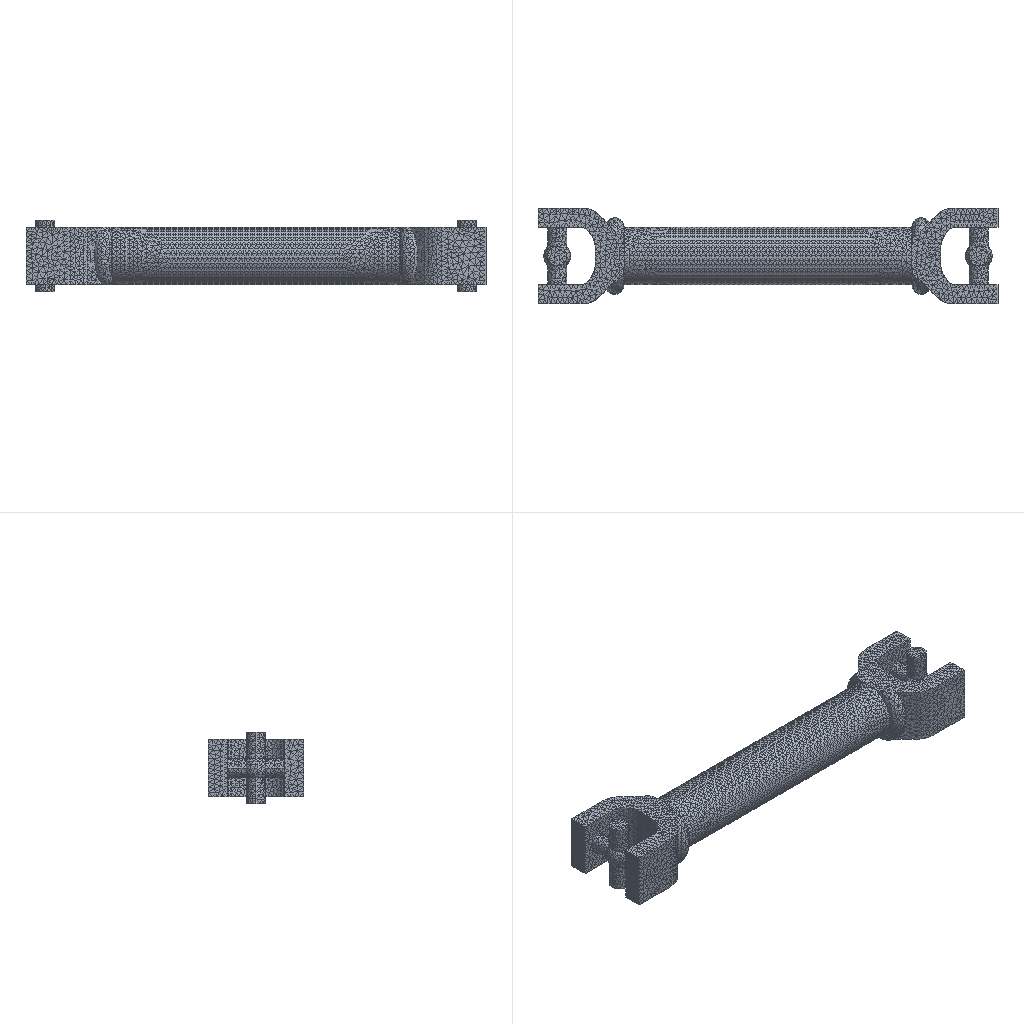Simulation study | ansys workbench
Set-up summary:
category,name,step,type,value,unit,region
solver,ansys_workbench
units,mm-N-s-tonne (MPa),,stated,"/units,MPA"
analysis,LS1,,modal,method=lanb; n_modes=10
load_step,LS1,LS1,modal
mesh,nodes,,,90919
mesh,elements,,,60202
element_type,SOLID187,,,58650
element_type,CONTA174,,,832
element_type,TARGE170,,,720
material,?,,E,240000,tonne s^-2 mm^-1
material,?,,nu,0.3
material,?,,density,6.9e-09,tonne mm^-3
material,16Mn?,,E,210000,tonne s^-2 mm^-1
material,16Mn?,,nu,0.3
material,16Mn?,,density,7.9e-09,tonne mm^-3
bc,Construct Remote Displacement,model,fixed,"[dofs=ROTX,ROTY,ROTZ,UX,UY,UZ n=12]",,node list
contact,Contact Region,,bonded (always),element=CONTA174
contact,Contact Region 2,,bonded (always),element=CONTA174
contact,contact 3,,bonded (always),element=CONTA174
contact,contact 4,,bonded (always),element=CONTA174
named_set,REMOTEDISPALL,,node,2
Ansys APDL input file, long lists of numbers shortened:
/batch
/config,noeldb,1     ! force off writing results to database
*get,_wallstrt,active,,time,wall
! ANSYS input file written by Workbench version 2021 R1
! File used for geometry attach:
/title,______--__ (C5)
! ****** Begin Custom Load Command Snippet ******
/COM, ACT Extensions:
/COM,     LSDYNA, 2021.1
/COM,
! ****** End   Custom Load Command Snippet ******
*DIM,_wb_ProjectScratch_dir,string,248
_wb_ProjectScratch_dir(1) = ''
*DIM,_wb_SolverFiles_dir,string,248
_wb_SolverFiles_dir(1) = ''
*DIM,_wb_userfiles_dir,string,248
_wb_userfiles_dir(1) = ''
/com,--- Data in consistent NMM units. See Solving Units in the help system for more information.
/units,MPA
/nopr
/wb,file,start              !  signify a WB generated input file
/prep7
! Turn off shape checking because checks already performed inside WB mesher.
! See help system for more information.
SHPP,OFF,,NOWARN
/nolist
etcon,set             ! allow ANSYS to choose best KEYOP's for 180x elements, resets any applicable keyopt to MAPDL defaults
/com,*********** Nodes for the whole assembly ***********
nblock,3,,100006
(1i9,3e20.9e3)
        1     7.600000000E+02    -2.000000000E+01     0.000000000E+00
! (90914 more lines like these left out)
-1
/com,*********** Nodes for all Remote Points ***********
nblock,3
(1i9,3e20.9e3)
    90916     7.400000000E+02     1.554312234E-14    -5.712370230E-07
    90917    -1.400000000E+02     1.402403685E-14    -1.421085472E-14
    90918     7.400000000E+02     1.402403685E-14     0.000000000E+00
    90919     7.400000000E+02     1.402403685E-14     0.000000000E+00
-1
/wb,elem,start            !  set before creation of elements
/com,*********** Elements for Body 1 "______|____2" ***********
et,1,187
eblock,19,solid,,52806
(19i9)
        1        1        1        1        0        0        0        0       10        0     5845    15480    21320    15698    17453    58957    61010    58952    58954
! (105611 more lines like these left out)
-1
/com,*********** Elements for Body 2 "______-0|____4" ***********
et,2,187
eblock,19,solid,,2922
(19i9)
        2        2        2        2        0        0        0        0       10        0     2923     5070     5085     5619     5377     6980     7061     6983     6981
! (5843 more lines like these left out)
-1
/com,*********** Elements for Body 3 "______-0|____4[2]" ***********
et,3,187
eblock,19,solid,,2922
(19i9)
        3        3        3        3        0        0        0        0       10        0        1      199      214      748      506     2109     2190     2112     2110
! (5843 more lines like these left out)
-1
/wb,elem,end               !  done creating elements
/com,*********** Send User Defined Coordinate System(s) ***********
csys,0
toffst,273.15,  ! Temperature offset from absolute zero
/com,*********** Set Reference Temperature ***********
tref,22.
/wb,mat,start              !  starting to send materials
/com,*********** Send Materials ***********
MP,DENS,1,6.9e-09,	! tonne mm^-3
MP,EX,1,240000,	! tonne s^-2 mm^-1
MP,NUXY,1,0.3,
MP,DENS,2,7.9e-09,	! tonne mm^-3
MP,EX,2,210000,	! tonne s^-2 mm^-1
MP,NUXY,2,0.3,
MP,DENS,3,7.9e-09,	! tonne mm^-3
MP,EX,3,210000,	! tonne s^-2 mm^-1
MP,NUXY,3,0.3,
/wb,mat,end                !  done sending materials
!************************* Model Summary ********************
!______|____2,	碳纤维合金钢,	matid,	1
!______-0|____4,	16Mn低合金钢,	matid,	2
!______-0|____4[2],	16Mn低合金钢,	matid,	3
!************************* End Model Summary ********************
! get the diagonal of the bounding box. Needed later for other things
*get,_xmin,node,,mnloc,x
*get,_ymin,node,,mnloc,y
*get,_zmin,node,,mnloc,z
*get,_xmax,node,,mxloc,x
*get,_ymax,node,,mxloc,y
*get,_zmax,node,,mxloc,z
_ASMDIAG=(_xmax-_xmin)*(_xmax-_xmin)+(_ymax-_ymin)*(_ymax-_ymin)+(_zmax-_zmin)*(_zmax-_zmin)
_ASMDIAG=SQRT(_ASMDIAG)
/wb,contact,start          !  starting to send contact
/com,*********** Create Contact "接触区域" ***********
/com,            Real Constant Set For Above Contact Is 5 & 4
*set,tid,5
*set,cid,4
r,tid
r,cid
et,tid,170
et,cid,174
eblock,10,,,160
(15i9)
    70895        5        5        5        0     9779     9788     9781     9781    21636    21646     9781    21635
! (159 more lines like these left out)
-1
eblock,10,,,160
(15i9)
    71055        4        4        4        0     9779     9788     9781     9781    21636    21646     9781    21635
! (159 more lines like these left out)
-1
eblock,10,,,200
(15i9)
    71215        4        5        4        0     4877     4884     4882     4882     5669     5706     4882     5668
! (199 more lines like these left out)
-1
eblock,10,,,200
(15i9)
    71415        5        4        5        0     4877     4884     4882     4882     5669     5706     4882     5668
! (199 more lines like these left out)
-1
keyo,cid,8,2               ! auto create asymmetric contact (from Program Controlled setting)
keyo,cid,10,0              ! adjust contact stiffness each NR iteration (from Program Controlled setting)
keyo,cid,12,5              ! bonded always
keyo,cid,18,1              ! small sliding turned on by application
keyo,cid,2,0               ! augmented Lagrange (from Program Controlled setting)
keyo,cid,4,0               ! on Gauss point (from Program Controlled setting)
keyo,cid,9,1               ! ignore initial gaps/penetration
keyo,cid,7,0               ! No Prediction
rmod,tid,3,10.      ! FKN
rmod,tid,5,0.       ! ICONT
rmod,tid,6,0.       ! PINB
rmod,tid,10,0.      ! CNOF
rmod,tid,12,0.      ! FKT
rmod,tid,36,31      ! WB DSID
rmod,cid,3,10.      ! FKN
rmod,cid,5,0.       ! ICONT
rmod,cid,6,0.       ! PINB
rmod,cid,10,0.      ! CNOF
rmod,cid,12,0.      ! FKT
rmod,cid,36,31      ! WB DSID
/com,*********** Create Contact "接触区域 2" ***********
/com,            Real Constant Set For Above Contact Is 7 & 6
*set,tid,7
*set,cid,6
r,tid
r,cid
et,tid,170
et,cid,174
eblock,10,,,160
(15i9)
    71615        7        7        7        0     9744     9752     9750     9750    21332    21399     9750    21331
! (159 more lines like these left out)
-1
eblock,10,,,160
(15i9)
    71775        6        6        6        0     9744     9752     9750     9750    21332    21399     9750    21331
! (159 more lines like these left out)
-1
eblock,10,,,200
(15i9)
    71935        6        7        6        0       57       55       64       64     1172     1173       64     1181
! (199 more lines like these left out)
-1
eblock,10,,,200
(15i9)
    72135        7        6        7        0       57       55       64       64     1172     1173       64     1181
! (199 more lines like these left out)
-1
keyo,cid,8,2               ! auto create asymmetric contact (from Program Controlled setting)
keyo,cid,10,0              ! adjust contact stiffness each NR iteration (from Program Controlled setting)
keyo,cid,12,5              ! bonded always
keyo,cid,18,1              ! small sliding turned on by application
keyo,cid,2,0               ! augmented Lagrange (from Program Controlled setting)
keyo,cid,4,0               ! on Gauss point (from Program Controlled setting)
keyo,cid,9,1               ! ignore initial gaps/penetration
keyo,cid,7,0               ! No Prediction
rmod,tid,3,10.      ! FKN
rmod,tid,5,0.       ! ICONT
rmod,tid,6,0.       ! PINB
rmod,tid,10,0.      ! CNOF
rmod,tid,12,0.      ! FKT
rmod,tid,36,34      ! WB DSID
rmod,cid,3,10.      ! FKN
rmod,cid,5,0.       ! ICONT
rmod,cid,6,0.       ! PINB
rmod,cid,10,0.      ! CNOF
rmod,cid,12,0.      ! FKT
rmod,cid,36,34      ! WB DSID
nsel,all
esel,all
/wb,contact,end            !  done creating contacts
/golist
/wb,load,start             !  starting to send loads
/com,*********** Create Remote Point "内部远程点 3" ***********
! -------- Remote Point Used by "远程位移" --------
*set,tid,9
*set,cid,8
et,cid,174
et,tid,170
keyo,tid,2,1               ! Don't fix the pilot node
keyo,tid,4,111111
keyo,cid,12,5              ! Bonded Contact
keyo,cid,4,1               ! Deformable RBE3 style load
keyo,cid,2,2               ! MPC style contact
eblock,10,,,56
(15i9)
    72335        8        8        8        0      148      437      149      149     1846     1851      149     1843
! (55 more lines like these left out)
-1
*set,_npilot,90918
_npilot135=_npilot
type,tid
mat ,cid
real,cid
tshape,pilo
en,72391,_npilot
tshape
/com,*********** Create Remote Point "内部远程点 3" ***********
! -------- Remote Point Used by "远程位移 2" --------
*set,tid,11
*set,cid,10
et,cid,174
et,tid,170
keyo,tid,2,1               ! Don't fix the pilot node
keyo,tid,4,111111
keyo,cid,12,5              ! Bonded Contact
keyo,cid,4,1               ! Deformable RBE3 style load
keyo,cid,2,2               ! MPC style contact
eblock,10,,,56
(15i9)
    72392       10       10       10        0     5019     5308     5020     5020     6717     6722     5020     6714
! (55 more lines like these left out)
-1
*set,_npilot,90919
_npilot152=_npilot
type,tid
mat ,cid
real,cid
tshape,pilo
en,72448,_npilot
tshape
/com,*********** Construct Remote Displacement ***********
*DIM,_loadvari134ux,TABLE,1,1,1,TIME,
! Time values
_loadvari134ux(1,0,1) = 1.
! Load values
_loadvari134ux(1,1,1) = 0.
*DIM,_loadvari134uy,TABLE,1,1,1,TIME,
! Time values
_loadvari134uy(1,0,1) = 1.
! Load values
_loadvari134uy(1,1,1) = 0.
*DIM,_loadvari134uz,TABLE,1,1,1,TIME,
! Time values
_loadvari134uz(1,0,1) = 1.
! Load values
_loadvari134uz(1,1,1) = 0.
*DIM,_loadvari134rotx,TABLE,1,1,1,TIME,
! Time values
_loadvari134rotx(1,0,1) = 1.
! Load values
_loadvari134rotx(1,1,1) = 0.
*DIM,_loadvari134roty,TABLE,1,1,1,TIME,
! Time values
_loadvari134roty(1,0,1) = 1.
! Load values
_loadvari134roty(1,1,1) = 0.
*DIM,_loadvari134rotz,TABLE,1,1,1,TIME,
! Time values
_loadvari134rotz(1,0,1) = 1.
! Load values
_loadvari134rotz(1,1,1) = 0.
/com,*********** Construct Remote Displacement ***********
*DIM,_loadvari151ux,TABLE,1,1,1,TIME,
! Time values
_loadvari151ux(1,0,1) = 1.
! Load values
_loadvari151ux(1,1,1) = 0.
*DIM,_loadvari151uy,TABLE,1,1,1,TIME,
! Time values
_loadvari151uy(1,0,1) = 1.
! Load values
_loadvari151uy(1,1,1) = 0.
*DIM,_loadvari151uz,TABLE,1,1,1,TIME,
! Time values
_loadvari151uz(1,0,1) = 1.
! Load values
_loadvari151uz(1,1,1) = 0.
*DIM,_loadvari151rotx,TABLE,1,1,1,TIME,
! Time values
_loadvari151rotx(1,0,1) = 1.
! Load values
_loadvari151rotx(1,1,1) = 0.
*DIM,_loadvari151roty,TABLE,1,1,1,TIME,
! Time values
_loadvari151roty(1,0,1) = 1.
! Load values
_loadvari151roty(1,1,1) = 0.
*DIM,_loadvari151rotz,TABLE,1,1,1,TIME,
! Time values
_loadvari151rotz(1,0,1) = 1.
! Load values
_loadvari151rotz(1,1,1) = 0.
d,90918,ux,%_loadvari134ux%
d,90918,uy,%_loadvari134uy%
d,90918,uz,%_loadvari134uz%
d,90918,rotx,%_loadvari134rotx%
d,90918,roty,%_loadvari134roty%
d,90918,rotz,%_loadvari134rotz%
d,90919,ux,%_loadvari151ux%
d,90919,uy,%_loadvari151uy%
d,90919,uz,%_loadvari151uz%
d,90919,rotx,%_loadvari151rotx%
d,90919,roty,%_loadvari151roty%
d,90919,rotz,%_loadvari151rotz%
/COM,*** Create a component for all remote displacements ***
CMBLOCK,REMOTEDISPALL,NODE,        2
(8i10)
     90918     90919
/gst,on,on
fini
*get,_numnode,node,0,count
*get,_numelem,elem,0,count
*get, _MAXELEMNUM, elem, 0, NUM, MAX
*get, _MAXNODENUM, node, 0, NUM, MAX
*get, _MAXELEMTYPE, etyp, 0, NUM, MAX
*get, _MAXREALCONST, real, 0, NUM, MAX
/go
/wb,load,end               !  done creating loads
/com,--- Number of total nodes = %_numnode%
/com,--- Number of contact elements = 1552
/com,--- Number of spring elements = 0
/com,--- Number of bearing elements = 0
/com,--- Number of solid elements = 58650
/com,--- Number of condensed parts = 0
/com,--- Number of total elements = %_numelem%
*get,_wallbsol,active,,time,wall
/solu
antype,2                   ! modal analysis
_thickRatio=  1     ! Ratio of thick parts in the model
modopt,lanb,10
outres,erase
outres,all,none
outres,nsol,all
outres,etmp,all
mxpand                    ! default expand in case of complex solution
dmpopt,esav,no
dmpopt,emat,no
dmpopt,full,no
! *********** WB SOLVE COMMAND ***********
! check interactive state
*get,ANSINTER_,active,,int
*if,ANSINTER_,ne,0,then
/eof
*endif
solve
/com *************** Write FE CONNECTORS *********
CEWRITE,file,ce,,INTE
*get,_nmodalsolproc,active,0,numcpu
fini
/nopr
*get,_numnode,node,0,count
*get,_numelem,elem,0,count
*get, _MAXELEMNUM, elem, 0, NUM, MAX
*get, _MAXNODENUM, node, 0, NUM, MAX,,,INTERNAL
*get, _MAXELEMTYPE, etyp, 0, NUM, MAX
*get, _MAXREALCONST, real, 0, NUM, MAX
/gopr
*get,_wallasol,active,,time,wall
/post1
/nopr
*dim,_direction,CHAR,6,1
_direction(1) = 'X'
_direction(2) = 'Y'
_direction(3) = 'Z'
_direction(4) = 'ROTX'
_direction(5) = 'ROTY'
_direction(6) = 'ROTZ'
*get,_lastLS,active,0,set,LSTP
*get,_beginset,active,0,set,nset,first,_lastLS
*get,_endset,active,0,set,nset,last,_lastLS
_nummodes = 0
*if,_endset,gt,0,then
_nummodes = _endset - _beginset + 1
*endif
*do,i_mode,1,_nummodes
   *do,j_component,1,6
			*get,PFACT_%i_mode%_%j_component%,MODE,%i_mode%,PFACT,,DIREC,_direction(%j_component%)
   *enddo
*enddo
*dim,_tmdirection,CHAR,6,1
_tmdirection(1) = 'X'
_tmdirection(2) = 'Y'
_tmdirection(3) = 'Z'
_tmdirection(4) = 'X'
_tmdirection(5) = 'Y'
_tmdirection(6) = 'Z'
*do,j_component,1,6
    *if,j_component,gt,3,then
        *get,TOTALMASS_%j_component%,ELEM,0,IOR,_tmdirection(%j_component%)
    *else
        *get,TOTALMASS_%j_component%,ELEM,0,MTOT,_tmdirection(%j_component%)
    *endif
*enddo
/gopr
xmlo,ENCODING,ISO-8859-1
xmlo,parm
/xml,parm,xml
fini
/gopr
*get,_walldone,active,,time,wall
_preptime=(_wallbsol-_wallstrt)*3600
_solvtime=(_wallasol-_wallbsol)*3600
_posttime=(_walldone-_wallasol)*3600
_totaltim=(_walldone-_wallstrt)*3600
*get,_dlbratio,active,0,solu,dlbr
*get,_combtime,active,0,solu,comb
/com,--- Total number of nodes = %_numnode%
/com,--- Total number of elements = %_numelem%
/com,--- Element load balance ratio = %_dlbratio%
/com,--- Time to combine distributed files = %_combtime%
/wb,file,end               ! done with WB generated input
Results summary:
result,analyses[0].index,,,1
result,analyses[0].system,,,SYS-2
result,analyses[0].deck,,,deck.dat
result,analyses[0].solve_status,,,completed
result,analyses[0].analysis_type,,,modal
result,analyses[0].physics,,,mechanical
result,analyses[0].unit_system,,,"NMM: mm, ton, N, s, mV, mA, degC"
result,analyses[0].n_sets,,,10
result,analyses[0].modal_frequencies_hz[1],,,295.624
result,analyses[0].modal_frequencies_hz[2],,,335.213
result,analyses[0].modal_frequencies_hz[3],,,458.34
result,analyses[0].modal_frequencies_hz[4],,,539.798
result,analyses[0].modal_frequencies_hz[5],,,726.321
result,analyses[0].modal_frequencies_hz[6],,,959.618
result,analyses[0].modal_frequencies_hz[7],,,1100.11
result,analyses[0].modal_frequencies_hz[8],,,1372.7
result,analyses[0].modal_frequencies_hz[9],,,1527.57
result,analyses[0].modal_frequencies_hz[10],,,1619.03
result,geometry_export[0][0],,,.step
result,geometry_export[0][1],,,ok
result,geometry_export[0][2],,,3